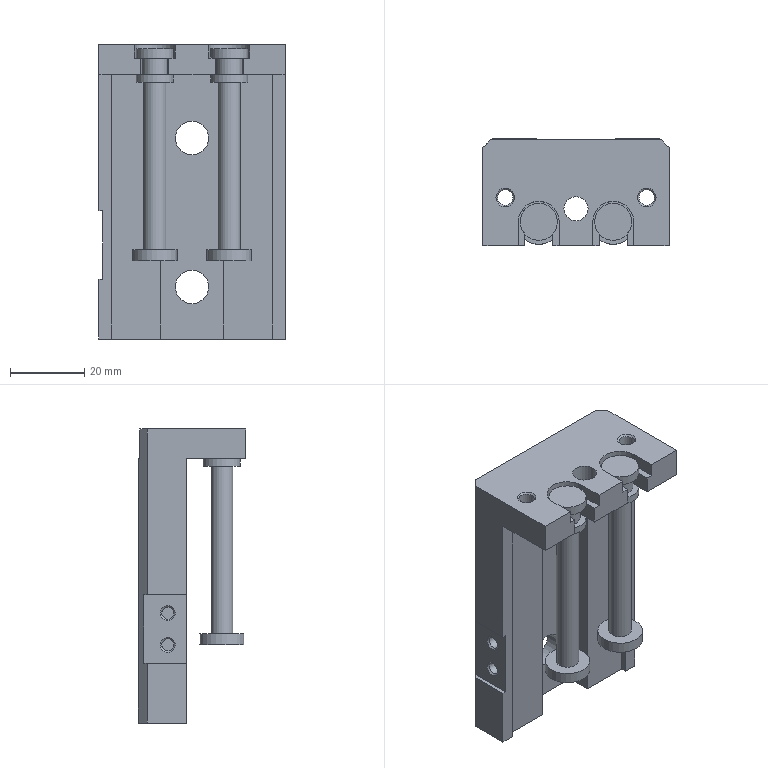Part | NX | 1 solid | 98 faces | box 50 x 29 x 79 mm | volume 45078 mm3 | plane 62 | cylinder 28 | cone 8 | commonest cylinder face diameters 3.242 x6 10 x4 4 x3 4.134 x2 6 x2 6.8 x2